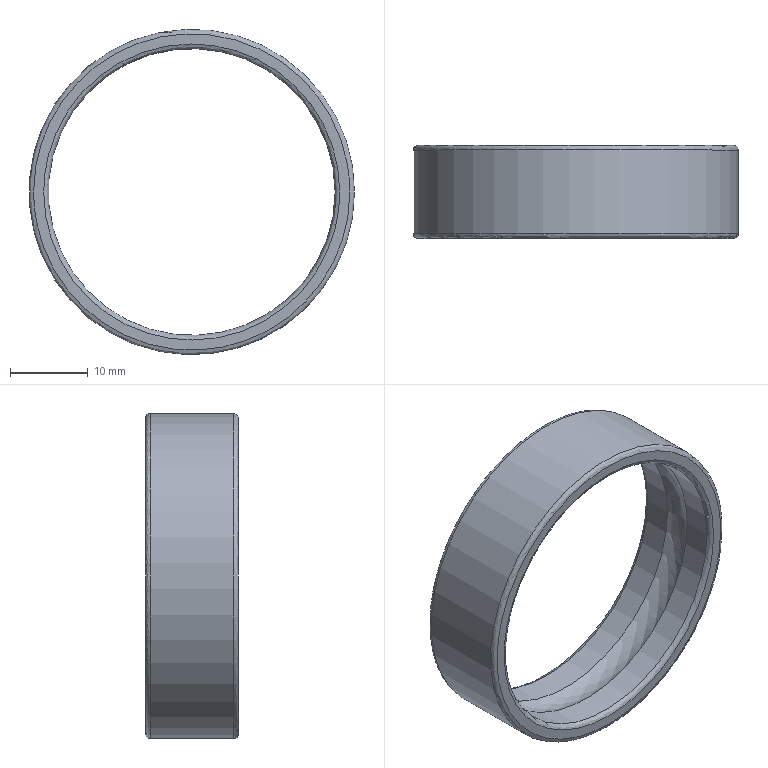Part | STEP file | BF-20_id1382_x_t | 1 solid | 10 faces | box 42 x 12 x 42 mm | volume 3541 mm3 | other 5 | cylinder 3 | plane 2 | commonest cylinder face diameters 37 x2 42 x1
STEP:
#1=CARTESIAN_POINT('',(0.,0.,0.));
#2=DIRECTION('',(0.,0.,1.));
#3=DIRECTION('',(1.,0.,0.));
#4=AXIS2_PLACEMENT_3D('',#1,#2,#3);
#5=CARTESIAN_POINT('',(-250.,-70.262,-165.5));
#6=VERTEX_POINT('',#5);
#7=CARTESIAN_POINT('',(-268.5,-70.262,-165.5));
#8=DIRECTION('',(0.,1.,0.));
#9=DIRECTION('',(1.,0.,0.));
#10=AXIS2_PLACEMENT_3D('',#7,#8,#9);
#11=CIRCLE('',#10,18.5);
#12=CARTESIAN_POINT('',(-253.,-72.064,-165.5));
#13=DIRECTION('',(0.,0.,1.));
#14=DIRECTION('',(1.,0.,0.));
#15=AXIS2_PLACEMENT_3D('',#12,#13,#14);
#16=CIRCLE('',#15,3.5);
#17=CARTESIAN_POINT('',(-268.5,-72.064,-165.5));
#18=DIRECTION('',(0.,-1.,0.));
#19=AXIS1_PLACEMENT('',#17,#18);
#20=SURFACE_OF_REVOLUTION('',#16,#19);
#21=CARTESIAN_POINT('',(6.283,6.824));
#22=DIRECTION('',(-1.,0.));
#23=VECTOR('',#22,1.);
#24=LINE('',#21,#23);
#25=(GEOMETRIC_REPRESENTATION_CONTEXT(2)PARAMETRIC_REPRESENTATION_CONTEXT()REPRESENTATION_CONTEXT('',''));
#26=DEFINITIONAL_REPRESENTATION('',(#24),#25);
#27=PCURVE('',#20,#26);
#28=CARTESIAN_POINT('',(-268.5,-80.904,-165.5));
#29=DIRECTION('',(0.,-1.,0.));
#30=DIRECTION('',(1.,0.,0.));
#31=AXIS2_PLACEMENT_3D('',#28,#29,#30);
#32=CYLINDRICAL_SURFACE('',#31,18.5);
#33=CARTESIAN_POINT('',(6.283,-10.642));
#34=DIRECTION('',(-1.,0.));
#35=VECTOR('',#34,1.);
#36=LINE('',#33,#35);
#37=(GEOMETRIC_REPRESENTATION_CONTEXT(2)PARAMETRIC_REPRESENTATION_CONTEXT()REPRESENTATION_CONTEXT('',''));
#38=DEFINITIONAL_REPRESENTATION('',(#36),#37);
#39=PCURVE('',#32,#38);
#40=SURFACE_CURVE('',#11,(#27,#39),.PCURVE_S1.);
#41=EDGE_CURVE('',#6,#6,#40,.T.);
#42=ORIENTED_EDGE('',*,*,#41,.T.);
#43=CARTESIAN_POINT('',(-250.,-73.867,-165.5));
#44=VERTEX_POINT('',#43);
#45=CARTESIAN_POINT('',(-250.,-73.867,-165.5));
#46=CARTESIAN_POINT('',(-249.675,-73.326,-165.5));
#47=CARTESIAN_POINT('',(-249.467,-72.715,-165.5));
#48=CARTESIAN_POINT('',(-249.395,-72.064,-165.5));
#49=CARTESIAN_POINT('',(-249.467,-71.414,-165.5));
#50=CARTESIAN_POINT('',(-249.675,-70.803,-165.5));
#51=CARTESIAN_POINT('',(-250.,-70.262,-165.5));
#52=B_SPLINE_CURVE_WITH_KNOTS('',6,(#45,#46,#47,#48,#49,#50,#51),.UNSPECIFIED.,.F.,.F.,(7,7),(-0.5411,0.5411),.PIECEWISE_BEZIER_KNOTS.);
#53=CARTESIAN_POINT('',(0.,6.283));
#54=DIRECTION('',(0.,1.));
#55=VECTOR('',#54,1.);
#56=LINE('',#53,#55);
#57=(GEOMETRIC_REPRESENTATION_CONTEXT(2)PARAMETRIC_REPRESENTATION_CONTEXT()REPRESENTATION_CONTEXT('',''));
#58=DEFINITIONAL_REPRESENTATION('',(#56),#57);
#59=PCURVE('',#20,#58);
#60=CARTESIAN_POINT('',(6.283,6.283));
#61=DIRECTION('',(0.,1.));
#62=VECTOR('',#61,1.);
#63=LINE('',#60,#62);
#64=(GEOMETRIC_REPRESENTATION_CONTEXT(2)PARAMETRIC_REPRESENTATION_CONTEXT()REPRESENTATION_CONTEXT('',''));
#65=DEFINITIONAL_REPRESENTATION('',(#63),#64);
#66=PCURVE('',#20,#65);
#67=SEAM_CURVE('',#52,(#59,#66),.PCURVE_S1.);
#68=EDGE_CURVE('',#44,#6,#67,.T.);
#69=ORIENTED_EDGE('',*,*,#68,.F.);
#70=CARTESIAN_POINT('',(-268.5,-73.867,-165.5));
#71=DIRECTION('',(0.,-1.,0.));
#72=DIRECTION('',(1.,0.,0.));
#73=AXIS2_PLACEMENT_3D('',#70,#71,#72);
#74=CIRCLE('',#73,18.5);
#75=CARTESIAN_POINT('',(0.,5.742));
#76=DIRECTION('',(1.,0.));
#77=VECTOR('',#76,1.);
#78=LINE('',#75,#77);
#79=(GEOMETRIC_REPRESENTATION_CONTEXT(2)PARAMETRIC_REPRESENTATION_CONTEXT()REPRESENTATION_CONTEXT('',''));
#80=DEFINITIONAL_REPRESENTATION('',(#78),#79);
#81=PCURVE('',#20,#80);
#82=CARTESIAN_POINT('',(-268.5,-80.904,-165.5));
#83=DIRECTION('',(0.,-1.,0.));
#84=DIRECTION('',(1.,0.,0.));
#85=AXIS2_PLACEMENT_3D('',#82,#83,#84);
#86=CYLINDRICAL_SURFACE('',#85,18.5);
#87=CARTESIAN_POINT('',(0.,-7.037));
#88=DIRECTION('',(1.,0.));
#89=VECTOR('',#88,1.);
#90=LINE('',#87,#89);
#91=(GEOMETRIC_REPRESENTATION_CONTEXT(2)PARAMETRIC_REPRESENTATION_CONTEXT()REPRESENTATION_CONTEXT('',''));
#92=DEFINITIONAL_REPRESENTATION('',(#90),#91);
#93=PCURVE('',#86,#92);
#94=SURFACE_CURVE('',#74,(#81,#93),.PCURVE_S1.);
#95=EDGE_CURVE('',#44,#44,#94,.T.);
#96=ORIENTED_EDGE('',*,*,#95,.T.);
#97=ORIENTED_EDGE('',*,*,#68,.T.);
#98=EDGE_LOOP('',(#42,#69,#96,#97));
#99=FACE_BOUND('',#98,.T.);
#100=ADVANCED_FACE('',(#99),#20,.T.);
#101=CARTESIAN_POINT('',(-250.,-66.664,-165.5));
#102=VERTEX_POINT('',#101);
#103=CARTESIAN_POINT('',(-268.5,-66.664,-165.5));
#104=DIRECTION('',(0.,-1.,0.));
#105=DIRECTION('',(1.,0.,0.));
#106=AXIS2_PLACEMENT_3D('',#103,#104,#105);
#107=CIRCLE('',#106,18.5);
#108=CARTESIAN_POINT('',(0.,-14.239));
#109=DIRECTION('',(1.,0.));
#110=VECTOR('',#109,1.);
#111=LINE('',#108,#110);
#112=(GEOMETRIC_REPRESENTATION_CONTEXT(2)PARAMETRIC_REPRESENTATION_CONTEXT()REPRESENTATION_CONTEXT('',''));
#113=DEFINITIONAL_REPRESENTATION('',(#111),#112);
#114=PCURVE('',#32,#113);
#115=CARTESIAN_POINT('',(-249.4,-66.664,-165.5));
#116=DIRECTION('',(0.,0.,1.));
#117=DIRECTION('',(1.,0.,0.));
#118=AXIS2_PLACEMENT_3D('',#115,#116,#117);
#119=CIRCLE('',#118,0.6);
#120=CARTESIAN_POINT('',(-268.5,-66.664,-165.5));
#121=DIRECTION('',(0.,-1.,0.));
#122=AXIS1_PLACEMENT('',#120,#121);
#123=SURFACE_OF_REVOLUTION('',#119,#122);
#124=CARTESIAN_POINT('',(0.,9.425));
#125=DIRECTION('',(1.,0.));
#126=VECTOR('',#125,1.);
#127=LINE('',#124,#126);
#128=(GEOMETRIC_REPRESENTATION_CONTEXT(2)PARAMETRIC_REPRESENTATION_CONTEXT()REPRESENTATION_CONTEXT('',''));
#129=DEFINITIONAL_REPRESENTATION('',(#127),#128);
#130=PCURVE('',#123,#129);
#131=SURFACE_CURVE('',#107,(#114,#130),.PCURVE_S1.);
#132=EDGE_CURVE('',#102,#102,#131,.T.);
#133=ORIENTED_EDGE('',*,*,#132,.T.);
#134=CARTESIAN_POINT('',(-250.,-66.664,-165.5));
#135=CARTESIAN_POINT('',(-250.,-70.262,-165.5));
#136=B_SPLINE_CURVE_WITH_KNOTS('',1,(#134,#135),.UNSPECIFIED.,.F.,.F.,(2,2),(-14.239,-10.642),.PIECEWISE_BEZIER_KNOTS.);
#137=CARTESIAN_POINT('',(6.283,0.));
#138=DIRECTION('',(0.,1.));
#139=VECTOR('',#138,1.);
#140=LINE('',#137,#139);
#141=(GEOMETRIC_REPRESENTATION_CONTEXT(2)PARAMETRIC_REPRESENTATION_CONTEXT()REPRESENTATION_CONTEXT('',''));
#142=DEFINITIONAL_REPRESENTATION('',(#140),#141);
#143=PCURVE('',#32,#142);
#144=CARTESIAN_POINT('',(0.,0.));
#145=DIRECTION('',(0.,1.));
#146=VECTOR('',#145,1.);
#147=LINE('',#144,#146);
#148=(GEOMETRIC_REPRESENTATION_CONTEXT(2)PARAMETRIC_REPRESENTATION_CONTEXT()REPRESENTATION_CONTEXT('',''));
#149=DEFINITIONAL_REPRESENTATION('',(#147),#148);
#150=PCURVE('',#32,#149);
#151=SEAM_CURVE('',#136,(#143,#150),.PCURVE_S1.);
#152=EDGE_CURVE('',#102,#6,#151,.T.);
#153=ORIENTED_EDGE('',*,*,#152,.T.);
#154=ORIENTED_EDGE('',*,*,#41,.T.);
#155=ORIENTED_EDGE('',*,*,#152,.F.);
#156=EDGE_LOOP('',(#133,#153,#154,#155));
#157=FACE_BOUND('',#156,.F.);
#158=ADVANCED_FACE('',(#157),#32,.F.);
#159=ORIENTED_EDGE('',*,*,#95,.T.);
#160=CARTESIAN_POINT('',(-250.,-77.464,-165.5));
#161=VERTEX_POINT('',#160);
#162=CARTESIAN_POINT('',(-250.,-73.867,-165.5));
#163=CARTESIAN_POINT('',(-250.,-77.464,-165.5));
#164=B_SPLINE_CURVE_WITH_KNOTS('',1,(#162,#163),.UNSPECIFIED.,.F.,.F.,(2,2),(-7.037,-3.439),.PIECEWISE_BEZIER_KNOTS.);
#165=CARTESIAN_POINT('',(6.283,0.));
#166=DIRECTION('',(0.,1.));
#167=VECTOR('',#166,1.);
#168=LINE('',#165,#167);
#169=(GEOMETRIC_REPRESENTATION_CONTEXT(2)PARAMETRIC_REPRESENTATION_CONTEXT()REPRESENTATION_CONTEXT('',''));
#170=DEFINITIONAL_REPRESENTATION('',(#168),#169);
#171=PCURVE('',#86,#170);
#172=CARTESIAN_POINT('',(0.,0.));
#173=DIRECTION('',(0.,1.));
#174=VECTOR('',#173,1.);
#175=LINE('',#172,#174);
#176=(GEOMETRIC_REPRESENTATION_CONTEXT(2)PARAMETRIC_REPRESENTATION_CONTEXT()REPRESENTATION_CONTEXT('',''));
#177=DEFINITIONAL_REPRESENTATION('',(#175),#176);
#178=PCURVE('',#86,#177);
#179=SEAM_CURVE('',#164,(#171,#178),.PCURVE_S1.);
#180=EDGE_CURVE('',#44,#161,#179,.T.);
#181=ORIENTED_EDGE('',*,*,#180,.T.);
#182=CARTESIAN_POINT('',(-268.5,-77.464,-165.5));
#183=DIRECTION('',(0.,1.,0.));
#184=DIRECTION('',(1.,0.,0.));
#185=AXIS2_PLACEMENT_3D('',#182,#183,#184);
#186=CIRCLE('',#185,18.5);
#187=CARTESIAN_POINT('',(6.283,-3.439));
#188=DIRECTION('',(-1.,0.));
#189=VECTOR('',#188,1.);
#190=LINE('',#187,#189);
#191=(GEOMETRIC_REPRESENTATION_CONTEXT(2)PARAMETRIC_REPRESENTATION_CONTEXT()REPRESENTATION_CONTEXT('',''));
#192=DEFINITIONAL_REPRESENTATION('',(#190),#191);
#193=PCURVE('',#86,#192);
#194=CARTESIAN_POINT('',(-249.4,-77.464,-165.5));
#195=DIRECTION('',(0.,0.,1.));
#196=DIRECTION('',(1.,0.,0.));
#197=AXIS2_PLACEMENT_3D('',#194,#195,#196);
#198=CIRCLE('',#197,0.6);
#199=CARTESIAN_POINT('',(-268.5,-77.464,-165.5));
#200=DIRECTION('',(0.,-1.,0.));
#201=AXIS1_PLACEMENT('',#199,#200);
#202=SURFACE_OF_REVOLUTION('',#198,#201);
#203=CARTESIAN_POINT('',(6.283,3.142));
#204=DIRECTION('',(-1.,0.));
#205=VECTOR('',#204,1.);
#206=LINE('',#203,#205);
#207=(GEOMETRIC_REPRESENTATION_CONTEXT(2)PARAMETRIC_REPRESENTATION_CONTEXT()REPRESENTATION_CONTEXT('',''));
#208=DEFINITIONAL_REPRESENTATION('',(#206),#207);
#209=PCURVE('',#202,#208);
#210=SURFACE_CURVE('',#186,(#193,#209),.PCURVE_S1.);
#211=EDGE_CURVE('',#161,#161,#210,.T.);
#212=ORIENTED_EDGE('',*,*,#211,.T.);
#213=ORIENTED_EDGE('',*,*,#180,.F.);
#214=EDGE_LOOP('',(#159,#181,#212,#213));
#215=FACE_BOUND('',#214,.F.);
#216=ADVANCED_FACE('',(#215),#86,.F.);
#217=CARTESIAN_POINT('',(-287.6,-66.064,-165.5));
#218=VERTEX_POINT('',#217);
#219=CARTESIAN_POINT('',(-249.4,-66.064,-165.5));
#220=VERTEX_POINT('',#219);
#221=CARTESIAN_POINT('',(-287.6,-66.064,-165.5));
#222=CARTESIAN_POINT('',(-287.6,-66.064,-127.3));
#223=CARTESIAN_POINT('',(-249.4,-66.064,-127.3));
#224=CARTESIAN_POINT('',(-249.4,-66.064,-165.5));
#225=(BOUNDED_CURVE()B_SPLINE_CURVE(3,(#221,#222,#223,#224),.UNSPECIFIED.,.F.,.F.)B_SPLINE_CURVE_WITH_KNOTS((4,4),(0.,1.),.PIECEWISE_BEZIER_KNOTS.)CURVE()GEOMETRIC_REPRESENTATION_ITEM()RATIONAL_B_SPLINE_CURVE((1.,0.3333,0.3333,1.))REPRESENTATION_ITEM(''));
#226=CARTESIAN_POINT('',(3.142,7.854));
#227=CARTESIAN_POINT('',(3.111,7.854));
#228=CARTESIAN_POINT('',(3.048,7.854));
#229=CARTESIAN_POINT('',(2.944,7.854));
#230=CARTESIAN_POINT('',(2.83,7.854));
#231=CARTESIAN_POINT('',(2.706,7.854));
#232=CARTESIAN_POINT('',(2.571,7.854));
#233=CARTESIAN_POINT('',(2.426,7.854));
#234=CARTESIAN_POINT('',(2.27,7.854));
#235=CARTESIAN_POINT('',(2.105,7.854));
#236=CARTESIAN_POINT('',(1.931,7.854));
#237=CARTESIAN_POINT('',(1.753,7.854));
#238=CARTESIAN_POINT('',(1.571,7.854));
#239=CARTESIAN_POINT('',(1.389,7.854));
#240=CARTESIAN_POINT('',(1.21,7.854));
#241=CARTESIAN_POINT('',(1.037,7.854));
#242=CARTESIAN_POINT('',(0.8717,7.854));
#243=CARTESIAN_POINT('',(0.7158,7.854));
#244=CARTESIAN_POINT('',(0.5703,7.854));
#245=CARTESIAN_POINT('',(0.4356,7.854));
#246=CARTESIAN_POINT('',(0.3115,7.854));
#247=CARTESIAN_POINT('',(0.1977,7.854));
#248=CARTESIAN_POINT('',(0.09367,7.854));
#249=CARTESIAN_POINT('',(0.0303,7.854));
#250=CARTESIAN_POINT('',(0.,7.854));
#251=B_SPLINE_CURVE_WITH_KNOTS('',3,(#226,#227,#228,#229,#230,#231,#232,#233,#234,#235,#236,#237,#238,#239,#240,#241,#242,#243,#244,#245,#246,#247,#248,#249,#250),.UNSPECIFIED.,.F.,.F.,(4,1,1,1,1,1,1,1,1,1,1,1,1,1,1,1,1,1,1,1,1,1,4),(0.,0.04545,0.09091,0.1364,0.1818,0.2273,0.2727,0.3182,0.3636,0.4091,0.4545,0.5,0.5455,0.5909,0.6364,0.6818,0.7273,0.7727,0.8182,0.8636,0.9091,0.9545,1.),.QUASI_UNIFORM_KNOTS.);
#252=(GEOMETRIC_REPRESENTATION_CONTEXT(2)PARAMETRIC_REPRESENTATION_CONTEXT()REPRESENTATION_CONTEXT('',''));
#253=DEFINITIONAL_REPRESENTATION('',(#251),#252);
#254=PCURVE('',#123,#253);
#255=CARTESIAN_POINT('',(-268.5,-66.064,-145.1));
#256=DIRECTION('',(0.,-1.,0.));
#257=DIRECTION('',(1.,0.,0.));
#258=AXIS2_PLACEMENT_3D('',#255,#256,#257);
#259=PLANE('',#258);
#260=CARTESIAN_POINT('',(-19.1,-20.4));
#261=CARTESIAN_POINT('',(-19.1,17.8));
#262=CARTESIAN_POINT('',(19.1,17.8));
#263=CARTESIAN_POINT('',(19.1,-20.4));
#264=(BOUNDED_CURVE()B_SPLINE_CURVE(3,(#260,#261,#262,#263),.UNSPECIFIED.,.F.,.F.)B_SPLINE_CURVE_WITH_KNOTS((4,4),(0.,1.),.PIECEWISE_BEZIER_KNOTS.)CURVE()GEOMETRIC_REPRESENTATION_ITEM()RATIONAL_B_SPLINE_CURVE((1.,0.3333,0.3333,1.))REPRESENTATION_ITEM(''));
#265=(GEOMETRIC_REPRESENTATION_CONTEXT(2)PARAMETRIC_REPRESENTATION_CONTEXT()REPRESENTATION_CONTEXT('',''));
#266=DEFINITIONAL_REPRESENTATION('',(#264),#265);
#267=PCURVE('',#259,#266);
#268=SURFACE_CURVE('',#225,(#254,#267),.PCURVE_S1.);
#269=EDGE_CURVE('',#218,#220,#268,.T.);
#270=ORIENTED_EDGE('',*,*,#269,.F.);
#271=CARTESIAN_POINT('',(-249.4,-66.064,-165.5));
#272=CARTESIAN_POINT('',(-249.4,-66.064,-203.7));
#273=CARTESIAN_POINT('',(-287.6,-66.064,-203.7));
#274=CARTESIAN_POINT('',(-287.6,-66.064,-165.5));
#275=(BOUNDED_CURVE()B_SPLINE_CURVE(3,(#271,#272,#273,#274),.UNSPECIFIED.,.F.,.F.)B_SPLINE_CURVE_WITH_KNOTS((4,4),(0.,1.),.PIECEWISE_BEZIER_KNOTS.)CURVE()GEOMETRIC_REPRESENTATION_ITEM()RATIONAL_B_SPLINE_CURVE((1.,0.3333,0.3333,1.))REPRESENTATION_ITEM(''));
#276=CARTESIAN_POINT('',(6.283,7.854));
#277=CARTESIAN_POINT('',(6.253,7.854));
#278=CARTESIAN_POINT('',(6.19,7.854));
#279=CARTESIAN_POINT('',(6.085,7.854));
#280=CARTESIAN_POINT('',(5.972,7.854));
#281=CARTESIAN_POINT('',(5.848,7.854));
#282=CARTESIAN_POINT('',(5.713,7.854));
#283=CARTESIAN_POINT('',(5.567,7.854));
#284=CARTESIAN_POINT('',(5.412,7.854));
#285=CARTESIAN_POINT('',(5.246,7.854));
#286=CARTESIAN_POINT('',(5.073,7.854));
#287=CARTESIAN_POINT('',(4.894,7.854));
#288=CARTESIAN_POINT('',(4.712,7.854));
#289=CARTESIAN_POINT('',(4.531,7.854));
#290=CARTESIAN_POINT('',(4.352,7.854));
#291=CARTESIAN_POINT('',(4.179,7.854));
#292=CARTESIAN_POINT('',(4.013,7.854));
#293=CARTESIAN_POINT('',(3.857,7.854));
#294=CARTESIAN_POINT('',(3.712,7.854));
#295=CARTESIAN_POINT('',(3.577,7.854));
#296=CARTESIAN_POINT('',(3.453,7.854));
#297=CARTESIAN_POINT('',(3.339,7.854));
#298=CARTESIAN_POINT('',(3.235,7.854));
#299=CARTESIAN_POINT('',(3.172,7.854));
#300=CARTESIAN_POINT('',(3.142,7.854));
#301=B_SPLINE_CURVE_WITH_KNOTS('',3,(#276,#277,#278,#279,#280,#281,#282,#283,#284,#285,#286,#287,#288,#289,#290,#291,#292,#293,#294,#295,#296,#297,#298,#299,#300),.UNSPECIFIED.,.F.,.F.,(4,1,1,1,1,1,1,1,1,1,1,1,1,1,1,1,1,1,1,1,1,1,4),(0.,0.04545,0.09091,0.1364,0.1818,0.2273,0.2727,0.3182,0.3636,0.4091,0.4545,0.5,0.5455,0.5909,0.6364,0.6818,0.7273,0.7727,0.8182,0.8636,0.9091,0.9545,1.),.QUASI_UNIFORM_KNOTS.);
#302=(GEOMETRIC_REPRESENTATION_CONTEXT(2)PARAMETRIC_REPRESENTATION_CONTEXT()REPRESENTATION_CONTEXT('',''));
#303=DEFINITIONAL_REPRESENTATION('',(#301),#302);
#304=PCURVE('',#123,#303);
#305=CARTESIAN_POINT('',(19.1,-20.4));
#306=CARTESIAN_POINT('',(19.1,-58.6));
#307=CARTESIAN_POINT('',(-19.1,-58.6));
#308=CARTESIAN_POINT('',(-19.1,-20.4));
#309=(BOUNDED_CURVE()B_SPLINE_CURVE(3,(#305,#306,#307,#308),.UNSPECIFIED.,.F.,.F.)B_SPLINE_CURVE_WITH_KNOTS((4,4),(0.,1.),.PIECEWISE_BEZIER_KNOTS.)CURVE()GEOMETRIC_REPRESENTATION_ITEM()RATIONAL_B_SPLINE_CURVE((1.,0.3333,0.3333,1.))REPRESENTATION_ITEM(''));
#310=(GEOMETRIC_REPRESENTATION_CONTEXT(2)PARAMETRIC_REPRESENTATION_CONTEXT()REPRESENTATION_CONTEXT('',''));
#311=DEFINITIONAL_REPRESENTATION('',(#309),#310);
#312=PCURVE('',#259,#311);
#313=SURFACE_CURVE('',#275,(#304,#312),.PCURVE_S1.);
#314=EDGE_CURVE('',#220,#218,#313,.T.);
#315=ORIENTED_EDGE('',*,*,#314,.F.);
#316=CARTESIAN_POINT('',(-249.4,-66.064,-165.5));
#317=CARTESIAN_POINT('',(-249.56,-66.064,-165.5));
#318=CARTESIAN_POINT('',(-249.717,-66.115,-165.5));
#319=CARTESIAN_POINT('',(-249.851,-66.213,-165.5));
#320=CARTESIAN_POINT('',(-249.949,-66.348,-165.5));
#321=CARTESIAN_POINT('',(-250.,-66.504,-165.5));
#322=CARTESIAN_POINT('',(-250.,-66.664,-165.5));
#323=(BOUNDED_CURVE()B_SPLINE_CURVE(6,(#316,#317,#318,#319,#320,#321,#322),.UNSPECIFIED.,.F.,.F.)B_SPLINE_CURVE_WITH_KNOTS((7,7),(1.571,3.142),.PIECEWISE_BEZIER_KNOTS.)CURVE()GEOMETRIC_REPRESENTATION_ITEM()RATIONAL_B_SPLINE_CURVE((1.031,1.01,0.9979,0.994,0.9979,1.01,1.031))REPRESENTATION_ITEM(''));
#324=CARTESIAN_POINT('',(6.283,6.283));
#325=DIRECTION('',(0.,1.));
#326=VECTOR('',#325,1.);
#327=LINE('',#324,#326);
#328=(GEOMETRIC_REPRESENTATION_CONTEXT(2)PARAMETRIC_REPRESENTATION_CONTEXT()REPRESENTATION_CONTEXT('',''));
#329=DEFINITIONAL_REPRESENTATION('',(#327),#328);
#330=PCURVE('',#123,#329);
#331=CARTESIAN_POINT('',(0.,6.283));
#332=DIRECTION('',(0.,1.));
#333=VECTOR('',#332,1.);
#334=LINE('',#331,#333);
#335=(GEOMETRIC_REPRESENTATION_CONTEXT(2)PARAMETRIC_REPRESENTATION_CONTEXT()REPRESENTATION_CONTEXT('',''));
#336=DEFINITIONAL_REPRESENTATION('',(#334),#335);
#337=PCURVE('',#123,#336);
#338=SEAM_CURVE('',#323,(#330,#337),.PCURVE_S1.);
#339=EDGE_CURVE('',#220,#102,#338,.T.);
#340=ORIENTED_EDGE('',*,*,#339,.T.);
#341=ORIENTED_EDGE('',*,*,#132,.F.);
#342=ORIENTED_EDGE('',*,*,#339,.F.);
#343=EDGE_LOOP('',(#270,#315,#340,#341,#342));
#344=FACE_BOUND('',#343,.F.);
#345=ADVANCED_FACE('',(#344),#123,.F.);
#346=ORIENTED_EDGE('',*,*,#211,.F.);
#347=CARTESIAN_POINT('',(-249.4,-78.064,-165.5));
#348=VERTEX_POINT('',#347);
#349=CARTESIAN_POINT('',(-250.,-77.464,-165.5));
#350=CARTESIAN_POINT('',(-250.,-77.625,-165.5));
#351=CARTESIAN_POINT('',(-249.949,-77.781,-165.5));
#352=CARTESIAN_POINT('',(-249.851,-77.916,-165.5));
#353=CARTESIAN_POINT('',(-249.717,-78.013,-165.5));
#354=CARTESIAN_POINT('',(-249.56,-78.064,-165.5));
#355=CARTESIAN_POINT('',(-249.4,-78.064,-165.5));
#356=(BOUNDED_CURVE()B_SPLINE_CURVE(6,(#349,#350,#351,#352,#353,#354,#355),.UNSPECIFIED.,.F.,.F.)B_SPLINE_CURVE_WITH_KNOTS((7,7),(3.142,4.712),.PIECEWISE_BEZIER_KNOTS.)CURVE()GEOMETRIC_REPRESENTATION_ITEM()RATIONAL_B_SPLINE_CURVE((1.031,1.01,0.9979,0.994,0.9979,1.01,1.031))REPRESENTATION_ITEM(''));
#357=CARTESIAN_POINT('',(6.283,0.));
#358=DIRECTION('',(0.,1.));
#359=VECTOR('',#358,1.);
#360=LINE('',#357,#359);
#361=(GEOMETRIC_REPRESENTATION_CONTEXT(2)PARAMETRIC_REPRESENTATION_CONTEXT()REPRESENTATION_CONTEXT('',''));
#362=DEFINITIONAL_REPRESENTATION('',(#360),#361);
#363=PCURVE('',#202,#362);
#364=CARTESIAN_POINT('',(0.,0.));
#365=DIRECTION('',(0.,1.));
#366=VECTOR('',#365,1.);
#367=LINE('',#364,#366);
#368=(GEOMETRIC_REPRESENTATION_CONTEXT(2)PARAMETRIC_REPRESENTATION_CONTEXT()REPRESENTATION_CONTEXT('',''));
#369=DEFINITIONAL_REPRESENTATION('',(#367),#368);
#370=PCURVE('',#202,#369);
#371=SEAM_CURVE('',#356,(#363,#370),.PCURVE_S1.);
#372=EDGE_CURVE('',#161,#348,#371,.T.);
#373=ORIENTED_EDGE('',*,*,#372,.T.);
#374=CARTESIAN_POINT('',(-287.6,-78.064,-165.5));
#375=VERTEX_POINT('',#374);
#376=CARTESIAN_POINT('',(-287.6,-78.064,-165.5));
#377=CARTESIAN_POINT('',(-287.6,-78.064,-203.7));
#378=CARTESIAN_POINT('',(-249.4,-78.064,-203.7));
#379=CARTESIAN_POINT('',(-249.4,-78.064,-165.5));
#380=(BOUNDED_CURVE()B_SPLINE_CURVE(3,(#376,#377,#378,#379),.UNSPECIFIED.,.F.,.F.)B_SPLINE_CURVE_WITH_KNOTS((4,4),(0.,1.),.PIECEWISE_BEZIER_KNOTS.)CURVE()GEOMETRIC_REPRESENTATION_ITEM()RATIONAL_B_SPLINE_CURVE((1.,0.3333,0.3333,1.))REPRESENTATION_ITEM(''));
#381=CARTESIAN_POINT('',(3.142,4.712));
#382=CARTESIAN_POINT('',(3.172,4.712));
#383=CARTESIAN_POINT('',(3.235,4.712));
#384=CARTESIAN_POINT('',(3.339,4.712));
#385=CARTESIAN_POINT('',(3.453,4.712));
#386=CARTESIAN_POINT('',(3.577,4.712));
#387=CARTESIAN_POINT('',(3.712,4.712));
#388=CARTESIAN_POINT('',(3.857,4.712));
#389=CARTESIAN_POINT('',(4.013,4.712));
#390=CARTESIAN_POINT('',(4.179,4.712));
#391=CARTESIAN_POINT('',(4.352,4.712));
#392=CARTESIAN_POINT('',(4.531,4.712));
#393=CARTESIAN_POINT('',(4.712,4.712));
#394=CARTESIAN_POINT('',(4.894,4.712));
#395=CARTESIAN_POINT('',(5.073,4.712));
#396=CARTESIAN_POINT('',(5.246,4.712));
#397=CARTESIAN_POINT('',(5.412,4.712));
#398=CARTESIAN_POINT('',(5.567,4.712));
#399=CARTESIAN_POINT('',(5.713,4.712));
#400=CARTESIAN_POINT('',(5.848,4.712));
#401=CARTESIAN_POINT('',(5.972,4.712));
#402=CARTESIAN_POINT('',(6.085,4.712));
#403=CARTESIAN_POINT('',(6.19,4.712));
#404=CARTESIAN_POINT('',(6.253,4.712));
#405=CARTESIAN_POINT('',(6.283,4.712));
#406=B_SPLINE_CURVE_WITH_KNOTS('',3,(#381,#382,#383,#384,#385,#386,#387,#388,#389,#390,#391,#392,#393,#394,#395,#396,#397,#398,#399,#400,#401,#402,#403,#404,#405),.UNSPECIFIED.,.F.,.F.,(4,1,1,1,1,1,1,1,1,1,1,1,1,1,1,1,1,1,1,1,1,1,4),(0.,0.04545,0.09091,0.1364,0.1818,0.2273,0.2727,0.3182,0.3636,0.4091,0.4545,0.5,0.5455,0.5909,0.6364,0.6818,0.7273,0.7727,0.8182,0.8636,0.9091,0.9545,1.),.QUASI_UNIFORM_KNOTS.);
#407=(GEOMETRIC_REPRESENTATION_CONTEXT(2)PARAMETRIC_REPRESENTATION_CONTEXT()REPRESENTATION_CONTEXT('',''));
#408=DEFINITIONAL_REPRESENTATION('',(#406),#407);
#409=PCURVE('',#202,#408);
#410=CARTESIAN_POINT('',(-268.5,-78.064,-145.1));
#411=DIRECTION('',(0.,1.,0.));
#412=DIRECTION('',(-1.,0.,0.));
#413=AXIS2_PLACEMENT_3D('',#410,#411,#412);
#414=PLANE('',#413);
#415=CARTESIAN_POINT('',(19.1,-20.4));
#416=CARTESIAN_POINT('',(19.1,-58.6));
#417=CARTESIAN_POINT('',(-19.1,-58.6));
#418=CARTESIAN_POINT('',(-19.1,-20.4));
#419=(BOUNDED_CURVE()B_SPLINE_CURVE(3,(#415,#416,#417,#418),.UNSPECIFIED.,.F.,.F.)B_SPLINE_CURVE_WITH_KNOTS((4,4),(0.,1.),.PIECEWISE_BEZIER_KNOTS.)CURVE()GEOMETRIC_REPRESENTATION_ITEM()RATIONAL_B_SPLINE_CURVE((1.,0.3333,0.3333,1.))REPRESENTATION_ITEM(''));
#420=(GEOMETRIC_REPRESENTATION_CONTEXT(2)PARAMETRIC_REPRESENTATION_CONTEXT()REPRESENTATION_CONTEXT('',''));
#421=DEFINITIONAL_REPRESENTATION('',(#419),#420);
#422=PCURVE('',#414,#421);
#423=SURFACE_CURVE('',#380,(#409,#422),.PCURVE_S1.);
#424=EDGE_CURVE('',#375,#348,#423,.T.);
#425=ORIENTED_EDGE('',*,*,#424,.F.);
#426=CARTESIAN_POINT('',(-249.4,-78.064,-165.5));
#427=CARTESIAN_POINT('',(-249.4,-78.064,-127.3));
#428=CARTESIAN_POINT('',(-287.6,-78.064,-127.3));
#429=CARTESIAN_POINT('',(-287.6,-78.064,-165.5));
#430=(BOUNDED_CURVE()B_SPLINE_CURVE(3,(#426,#427,#428,#429),.UNSPECIFIED.,.F.,.F.)B_SPLINE_CURVE_WITH_KNOTS((4,4),(0.,1.),.PIECEWISE_BEZIER_KNOTS.)CURVE()GEOMETRIC_REPRESENTATION_ITEM()RATIONAL_B_SPLINE_CURVE((1.,0.3333,0.3333,1.))REPRESENTATION_ITEM(''));
#431=CARTESIAN_POINT('',(0.,4.712));
#432=CARTESIAN_POINT('',(0.0303,4.712));
#433=CARTESIAN_POINT('',(0.09367,4.712));
#434=CARTESIAN_POINT('',(0.1977,4.712));
#435=CARTESIAN_POINT('',(0.3115,4.712));
#436=CARTESIAN_POINT('',(0.4356,4.712));
#437=CARTESIAN_POINT('',(0.5703,4.712));
#438=CARTESIAN_POINT('',(0.7158,4.712));
#439=CARTESIAN_POINT('',(0.8717,4.712));
#440=CARTESIAN_POINT('',(1.037,4.712));
#441=CARTESIAN_POINT('',(1.21,4.712));
#442=CARTESIAN_POINT('',(1.389,4.712));
#443=CARTESIAN_POINT('',(1.571,4.712));
#444=CARTESIAN_POINT('',(1.753,4.712));
#445=CARTESIAN_POINT('',(1.931,4.712));
#446=CARTESIAN_POINT('',(2.105,4.712));
#447=CARTESIAN_POINT('',(2.27,4.712));
#448=CARTESIAN_POINT('',(2.426,4.712));
#449=CARTESIAN_POINT('',(2.571,4.712));
#450=CARTESIAN_POINT('',(2.706,4.712));
#451=CARTESIAN_POINT('',(2.83,4.712));
#452=CARTESIAN_POINT('',(2.944,4.712));
#453=CARTESIAN_POINT('',(3.048,4.712));
#454=CARTESIAN_POINT('',(3.111,4.712));
#455=CARTESIAN_POINT('',(3.142,4.712));
#456=B_SPLINE_CURVE_WITH_KNOTS('',3,(#431,#432,#433,#434,#435,#436,#437,#438,#439,#440,#441,#442,#443,#444,#445,#446,#447,#448,#449,#450,#451,#452,#453,#454,#455),.UNSPECIFIED.,.F.,.F.,(4,1,1,1,1,1,1,1,1,1,1,1,1,1,1,1,1,1,1,1,1,1,4),(0.,0.04545,0.09091,0.1364,0.1818,0.2273,0.2727,0.3182,0.3636,0.4091,0.4545,0.5,0.5455,0.5909,0.6364,0.6818,0.7273,0.7727,0.8182,0.8636,0.9091,0.9545,1.),.QUASI_UNIFORM_KNOTS.);
#457=(GEOMETRIC_REPRESENTATION_CONTEXT(2)PARAMETRIC_REPRESENTATION_CONTEXT()REPRESENTATION_CONTEXT('',''));
#458=DEFINITIONAL_REPRESENTATION('',(#456),#457);
#459=PCURVE('',#202,#458);
#460=CARTESIAN_POINT('',(-19.1,-20.4));
#461=CARTESIAN_POINT('',(-19.1,17.8));
#462=CARTESIAN_POINT('',(19.1,17.8));
#463=CARTESIAN_POINT('',(19.1,-20.4));
#464=(BOUNDED_CURVE()B_SPLINE_CURVE(3,(#460,#461,#462,#463),.UNSPECIFIED.,.F.,.F.)B_SPLINE_CURVE_WITH_KNOTS((4,4),(0.,1.),.PIECEWISE_BEZIER_KNOTS.)CURVE()GEOMETRIC_REPRESENTATION_ITEM()RATIONAL_B_SPLINE_CURVE((1.,0.3333,0.3333,1.))REPRESENTATION_ITEM(''));
#465=(GEOMETRIC_REPRESENTATION_CONTEXT(2)PARAMETRIC_REPRESENTATION_CONTEXT()REPRESENTATION_CONTEXT('',''));
#466=DEFINITIONAL_REPRESENTATION('',(#464),#465);
#467=PCURVE('',#414,#466);
#468=SURFACE_CURVE('',#430,(#459,#467),.PCURVE_S1.);
#469=EDGE_CURVE('',#348,#375,#468,.T.);
#470=ORIENTED_EDGE('',*,*,#469,.F.);
#471=ORIENTED_EDGE('',*,*,#372,.F.);
#472=EDGE_LOOP('',(#346,#373,#425,#470,#471));
#473=FACE_BOUND('',#472,.F.);
#474=ADVANCED_FACE('',(#473),#202,.F.);
#475=ORIENTED_EDGE('',*,*,#314,.F.);
#476=ORIENTED_EDGE('',*,*,#269,.F.);
#477=EDGE_LOOP('',(#475,#476));
#478=FACE_BOUND('',#477,.T.);
#479=CARTESIAN_POINT('',(-288.9,-66.064,-165.5));
#480=VERTEX_POINT('',#479);
#481=CARTESIAN_POINT('',(-248.1,-66.064,-165.5));
#482=VERTEX_POINT('',#481);
#483=CARTESIAN_POINT('',(-288.9,-66.064,-165.5));
#484=CARTESIAN_POINT('',(-288.9,-66.064,-206.3));
#485=CARTESIAN_POINT('',(-248.1,-66.064,-206.3));
#486=CARTESIAN_POINT('',(-248.1,-66.064,-165.5));
#487=(BOUNDED_CURVE()B_SPLINE_CURVE(3,(#483,#484,#485,#486),.UNSPECIFIED.,.F.,.F.)B_SPLINE_CURVE_WITH_KNOTS((4,4),(0.,1.),.PIECEWISE_BEZIER_KNOTS.)CURVE()GEOMETRIC_REPRESENTATION_ITEM()RATIONAL_B_SPLINE_CURVE((1.,0.3333,0.3333,1.))REPRESENTATION_ITEM(''));
#488=CARTESIAN_POINT('',(-20.4,-20.4));
#489=CARTESIAN_POINT('',(-20.4,-61.2));
#490=CARTESIAN_POINT('',(20.4,-61.2));
#491=CARTESIAN_POINT('',(20.4,-20.4));
#492=(BOUNDED_CURVE()B_SPLINE_CURVE(3,(#488,#489,#490,#491),.UNSPECIFIED.,.F.,.F.)B_SPLINE_CURVE_WITH_KNOTS((4,4),(0.,1.),.PIECEWISE_BEZIER_KNOTS.)CURVE()GEOMETRIC_REPRESENTATION_ITEM()RATIONAL_B_SPLINE_CURVE((1.,0.3333,0.3333,1.))REPRESENTATION_ITEM(''));
#493=(GEOMETRIC_REPRESENTATION_CONTEXT(2)PARAMETRIC_REPRESENTATION_CONTEXT()REPRESENTATION_CONTEXT('',''));
#494=DEFINITIONAL_REPRESENTATION('',(#492),#493);
#495=PCURVE('',#259,#494);
#496=CARTESIAN_POINT('',(-248.1,-66.664,-165.5));
#497=DIRECTION('',(0.,0.,1.));
#498=DIRECTION('',(1.,0.,0.));
#499=AXIS2_PLACEMENT_3D('',#496,#497,#498);
#500=CIRCLE('',#499,0.6);
#501=CARTESIAN_POINT('',(-268.5,-66.664,-165.5));
#502=DIRECTION('',(0.,-1.,0.));
#503=AXIS1_PLACEMENT('',#501,#502);
#504=SURFACE_OF_REVOLUTION('',#500,#503);
#505=CARTESIAN_POINT('',(3.142,7.854));
#506=CARTESIAN_POINT('',(3.172,7.854));
#507=CARTESIAN_POINT('',(3.235,7.854));
#508=CARTESIAN_POINT('',(3.339,7.854));
#509=CARTESIAN_POINT('',(3.453,7.854));
#510=CARTESIAN_POINT('',(3.577,7.854));
#511=CARTESIAN_POINT('',(3.712,7.854));
#512=CARTESIAN_POINT('',(3.857,7.854));
#513=CARTESIAN_POINT('',(4.013,7.854));
#514=CARTESIAN_POINT('',(4.179,7.854));
#515=CARTESIAN_POINT('',(4.352,7.854));
#516=CARTESIAN_POINT('',(4.531,7.854));
#517=CARTESIAN_POINT('',(4.712,7.854));
#518=CARTESIAN_POINT('',(4.894,7.854));
#519=CARTESIAN_POINT('',(5.073,7.854));
#520=CARTESIAN_POINT('',(5.246,7.854));
#521=CARTESIAN_POINT('',(5.412,7.854));
#522=CARTESIAN_POINT('',(5.567,7.854));
#523=CARTESIAN_POINT('',(5.713,7.854));
#524=CARTESIAN_POINT('',(5.848,7.854));
#525=CARTESIAN_POINT('',(5.972,7.854));
#526=CARTESIAN_POINT('',(6.085,7.854));
#527=CARTESIAN_POINT('',(6.19,7.854));
#528=CARTESIAN_POINT('',(6.253,7.854));
#529=CARTESIAN_POINT('',(6.283,7.854));
#530=B_SPLINE_CURVE_WITH_KNOTS('',3,(#505,#506,#507,#508,#509,#510,#511,#512,#513,#514,#515,#516,#517,#518,#519,#520,#521,#522,#523,#524,#525,#526,#527,#528,#529),.UNSPECIFIED.,.F.,.F.,(4,1,1,1,1,1,1,1,1,1,1,1,1,1,1,1,1,1,1,1,1,1,4),(0.,0.04545,0.09091,0.1364,0.1818,0.2273,0.2727,0.3182,0.3636,0.4091,0.4545,0.5,0.5455,0.5909,0.6364,0.6818,0.7273,0.7727,0.8182,0.8636,0.9091,0.9545,1.),.QUASI_UNIFORM_KNOTS.);
#531=(GEOMETRIC_REPRESENTATION_CONTEXT(2)PARAMETRIC_REPRESENTATION_CONTEXT()REPRESENTATION_CONTEXT('',''));
#532=DEFINITIONAL_REPRESENTATION('',(#530),#531);
#533=PCURVE('',#504,#532);
#534=SURFACE_CURVE('',#487,(#495,#533),.PCURVE_S1.);
#535=EDGE_CURVE('',#480,#482,#534,.T.);
#536=ORIENTED_EDGE('',*,*,#535,.F.);
#537=CARTESIAN_POINT('',(-248.1,-66.064,-165.5));
#538=CARTESIAN_POINT('',(-248.1,-66.064,-124.7));
#539=CARTESIAN_POINT('',(-288.9,-66.064,-124.7));
#540=CARTESIAN_POINT('',(-288.9,-66.064,-165.5));
#541=(BOUNDED_CURVE()B_SPLINE_CURVE(3,(#537,#538,#539,#540),.UNSPECIFIED.,.F.,.F.)B_SPLINE_CURVE_WITH_KNOTS((4,4),(0.,1.),.PIECEWISE_BEZIER_KNOTS.)CURVE()GEOMETRIC_REPRESENTATION_ITEM()RATIONAL_B_SPLINE_CURVE((1.,0.3333,0.3333,1.))REPRESENTATION_ITEM(''));
#542=CARTESIAN_POINT('',(20.4,-20.4));
#543=CARTESIAN_POINT('',(20.4,20.4));
#544=CARTESIAN_POINT('',(-20.4,20.4));
#545=CARTESIAN_POINT('',(-20.4,-20.4));
#546=(BOUNDED_CURVE()B_SPLINE_CURVE(3,(#542,#543,#544,#545),.UNSPECIFIED.,.F.,.F.)B_SPLINE_CURVE_WITH_KNOTS((4,4),(0.,1.),.PIECEWISE_BEZIER_KNOTS.)CURVE()GEOMETRIC_REPRESENTATION_ITEM()RATIONAL_B_SPLINE_CURVE((1.,0.3333,0.3333,1.))REPRESENTATION_ITEM(''));
#547=(GEOMETRIC_REPRESENTATION_CONTEXT(2)PARAMETRIC_REPRESENTATION_CONTEXT()REPRESENTATION_CONTEXT('',''));
#548=DEFINITIONAL_REPRESENTATION('',(#546),#547);
#549=PCURVE('',#259,#548);
#550=CARTESIAN_POINT('',(0.,7.854));
#551=CARTESIAN_POINT('',(0.0303,7.854));
#552=CARTESIAN_POINT('',(0.09367,7.854));
#553=CARTESIAN_POINT('',(0.1977,7.854));
#554=CARTESIAN_POINT('',(0.3115,7.854));
#555=CARTESIAN_POINT('',(0.4356,7.854));
#556=CARTESIAN_POINT('',(0.5703,7.854));
#557=CARTESIAN_POINT('',(0.7158,7.854));
#558=CARTESIAN_POINT('',(0.8717,7.854));
#559=CARTESIAN_POINT('',(1.037,7.854));
#560=CARTESIAN_POINT('',(1.21,7.854));
#561=CARTESIAN_POINT('',(1.389,7.854));
#562=CARTESIAN_POINT('',(1.571,7.854));
#563=CARTESIAN_POINT('',(1.753,7.854));
#564=CARTESIAN_POINT('',(1.931,7.854));
#565=CARTESIAN_POINT('',(2.105,7.854));
#566=CARTESIAN_POINT('',(2.27,7.854));
#567=CARTESIAN_POINT('',(2.426,7.854));
#568=CARTESIAN_POINT('',(2.571,7.854));
#569=CARTESIAN_POINT('',(2.706,7.854));
#570=CARTESIAN_POINT('',(2.83,7.854));
#571=CARTESIAN_POINT('',(2.944,7.854));
#572=CARTESIAN_POINT('',(3.048,7.854));
#573=CARTESIAN_POINT('',(3.111,7.854));
#574=CARTESIAN_POINT('',(3.142,7.854));
#575=B_SPLINE_CURVE_WITH_KNOTS('',3,(#550,#551,#552,#553,#554,#555,#556,#557,#558,#559,#560,#561,#562,#563,#564,#565,#566,#567,#568,#569,#570,#571,#572,#573,#574),.UNSPECIFIED.,.F.,.F.,(4,1,1,1,1,1,1,1,1,1,1,1,1,1,1,1,1,1,1,1,1,1,4),(0.,0.04545,0.09091,0.1364,0.1818,0.2273,0.2727,0.3182,0.3636,0.4091,0.4545,0.5,0.5455,0.5909,0.6364,0.6818,0.7273,0.7727,0.8182,0.8636,0.9091,0.9545,1.),.QUASI_UNIFORM_KNOTS.);
#576=(GEOMETRIC_REPRESENTATION_CONTEXT(2)PARAMETRIC_REPRESENTATION_CONTEXT()REPRESENTATION_CONTEXT('',''));
#577=DEFINITIONAL_REPRESENTATION('',(#575),#576);
#578=PCURVE('',#504,#577);
#579=SURFACE_CURVE('',#541,(#549,#578),.PCURVE_S1.);
#580=EDGE_CURVE('',#482,#480,#579,.T.);
#581=ORIENTED_EDGE('',*,*,#580,.F.);
#582=EDGE_LOOP('',(#536,#581));
#583=FACE_BOUND('',#582,.T.);
#584=ADVANCED_FACE('',(#478,#583),#259,.F.);
#585=CARTESIAN_POINT('',(-248.1,-78.064,-165.5));
#586=VERTEX_POINT('',#585);
#587=CARTESIAN_POINT('',(-288.9,-78.064,-165.5));
#588=VERTEX_POINT('',#587);
#589=CARTESIAN_POINT('',(-248.1,-78.064,-165.5));
#590=CARTESIAN_POINT('',(-248.1,-78.064,-206.3));
#591=CARTESIAN_POINT('',(-288.9,-78.064,-206.3));
#592=CARTESIAN_POINT('',(-288.9,-78.064,-165.5));
#593=(BOUNDED_CURVE()B_SPLINE_CURVE(3,(#589,#590,#591,#592),.UNSPECIFIED.,.F.,.F.)B_SPLINE_CURVE_WITH_KNOTS((4,4),(0.,1.),.PIECEWISE_BEZIER_KNOTS.)CURVE()GEOMETRIC_REPRESENTATION_ITEM()RATIONAL_B_SPLINE_CURVE((1.,0.3333,0.3333,1.))REPRESENTATION_ITEM(''));
#594=CARTESIAN_POINT('',(-20.4,-20.4));
#595=CARTESIAN_POINT('',(-20.4,-61.2));
#596=CARTESIAN_POINT('',(20.4,-61.2));
#597=CARTESIAN_POINT('',(20.4,-20.4));
#598=(BOUNDED_CURVE()B_SPLINE_CURVE(3,(#594,#595,#596,#597),.UNSPECIFIED.,.F.,.F.)B_SPLINE_CURVE_WITH_KNOTS((4,4),(0.,1.),.PIECEWISE_BEZIER_KNOTS.)CURVE()GEOMETRIC_REPRESENTATION_ITEM()RATIONAL_B_SPLINE_CURVE((1.,0.3333,0.3333,1.))REPRESENTATION_ITEM(''));
#599=(GEOMETRIC_REPRESENTATION_CONTEXT(2)PARAMETRIC_REPRESENTATION_CONTEXT()REPRESENTATION_CONTEXT('',''));
#600=DEFINITIONAL_REPRESENTATION('',(#598),#599);
#601=PCURVE('',#414,#600);
#602=CARTESIAN_POINT('',(-248.1,-77.464,-165.5));
#603=DIRECTION('',(0.,0.,1.));
#604=DIRECTION('',(1.,0.,0.));
#605=AXIS2_PLACEMENT_3D('',#602,#603,#604);
#606=CIRCLE('',#605,0.6);
#607=CARTESIAN_POINT('',(-268.5,-77.464,-165.5));
#608=DIRECTION('',(0.,-1.,0.));
#609=AXIS1_PLACEMENT('',#607,#608);
#610=SURFACE_OF_REVOLUTION('',#606,#609);
#611=CARTESIAN_POINT('',(6.283,4.712));
#612=CARTESIAN_POINT('',(6.253,4.712));
#613=CARTESIAN_POINT('',(6.19,4.712));
#614=CARTESIAN_POINT('',(6.085,4.712));
#615=CARTESIAN_POINT('',(5.972,4.712));
#616=CARTESIAN_POINT('',(5.848,4.712));
#617=CARTESIAN_POINT('',(5.713,4.712));
#618=CARTESIAN_POINT('',(5.567,4.712));
#619=CARTESIAN_POINT('',(5.412,4.712));
#620=CARTESIAN_POINT('',(5.246,4.712));
#621=CARTESIAN_POINT('',(5.073,4.712));
#622=CARTESIAN_POINT('',(4.894,4.712));
#623=CARTESIAN_POINT('',(4.712,4.712));
#624=CARTESIAN_POINT('',(4.531,4.712));
#625=CARTESIAN_POINT('',(4.352,4.712));
#626=CARTESIAN_POINT('',(4.179,4.712));
#627=CARTESIAN_POINT('',(4.013,4.712));
#628=CARTESIAN_POINT('',(3.857,4.712));
#629=CARTESIAN_POINT('',(3.712,4.712));
#630=CARTESIAN_POINT('',(3.577,4.712));
#631=CARTESIAN_POINT('',(3.453,4.712));
#632=CARTESIAN_POINT('',(3.339,4.712));
#633=CARTESIAN_POINT('',(3.235,4.712));
#634=CARTESIAN_POINT('',(3.172,4.712));
#635=CARTESIAN_POINT('',(3.142,4.712));
#636=B_SPLINE_CURVE_WITH_KNOTS('',3,(#611,#612,#613,#614,#615,#616,#617,#618,#619,#620,#621,#622,#623,#624,#625,#626,#627,#628,#629,#630,#631,#632,#633,#634,#635),.UNSPECIFIED.,.F.,.F.,(4,1,1,1,1,1,1,1,1,1,1,1,1,1,1,1,1,1,1,1,1,1,4),(0.,0.04545,0.09091,0.1364,0.1818,0.2273,0.2727,0.3182,0.3636,0.4091,0.4545,0.5,0.5455,0.5909,0.6364,0.6818,0.7273,0.7727,0.8182,0.8636,0.9091,0.9545,1.),.QUASI_UNIFORM_KNOTS.);
#637=(GEOMETRIC_REPRESENTATION_CONTEXT(2)PARAMETRIC_REPRESENTATION_CONTEXT()REPRESENTATION_CONTEXT('',''));
#638=DEFINITIONAL_REPRESENTATION('',(#636),#637);
#639=PCURVE('',#610,#638);
#640=SURFACE_CURVE('',#593,(#601,#639),.PCURVE_S1.);
#641=EDGE_CURVE('',#586,#588,#640,.T.);
#642=ORIENTED_EDGE('',*,*,#641,.F.);
#643=CARTESIAN_POINT('',(-288.9,-78.064,-165.5));
#644=CARTESIAN_POINT('',(-288.9,-78.064,-124.7));
#645=CARTESIAN_POINT('',(-248.1,-78.064,-124.7));
#646=CARTESIAN_POINT('',(-248.1,-78.064,-165.5));
#647=(BOUNDED_CURVE()B_SPLINE_CURVE(3,(#643,#644,#645,#646),.UNSPECIFIED.,.F.,.F.)B_SPLINE_CURVE_WITH_KNOTS((4,4),(0.,1.),.PIECEWISE_BEZIER_KNOTS.)CURVE()GEOMETRIC_REPRESENTATION_ITEM()RATIONAL_B_SPLINE_CURVE((1.,0.3333,0.3333,1.))REPRESENTATION_ITEM(''));
#648=CARTESIAN_POINT('',(20.4,-20.4));
#649=CARTESIAN_POINT('',(20.4,20.4));
#650=CARTESIAN_POINT('',(-20.4,20.4));
#651=CARTESIAN_POINT('',(-20.4,-20.4));
#652=(BOUNDED_CURVE()B_SPLINE_CURVE(3,(#648,#649,#650,#651),.UNSPECIFIED.,.F.,.F.)B_SPLINE_CURVE_WITH_KNOTS((4,4),(0.,1.),.PIECEWISE_BEZIER_KNOTS.)CURVE()GEOMETRIC_REPRESENTATION_ITEM()RATIONAL_B_SPLINE_CURVE((1.,0.3333,0.3333,1.))REPRESENTATION_ITEM(''));
#653=(GEOMETRIC_REPRESENTATION_CONTEXT(2)PARAMETRIC_REPRESENTATION_CONTEXT()REPRESENTATION_CONTEXT('',''));
#654=DEFINITIONAL_REPRESENTATION('',(#652),#653);
#655=PCURVE('',#414,#654);
#656=CARTESIAN_POINT('',(3.142,4.712));
#657=CARTESIAN_POINT('',(3.111,4.712));
#658=CARTESIAN_POINT('',(3.048,4.712));
#659=CARTESIAN_POINT('',(2.944,4.712));
#660=CARTESIAN_POINT('',(2.83,4.712));
#661=CARTESIAN_POINT('',(2.706,4.712));
#662=CARTESIAN_POINT('',(2.571,4.712));
#663=CARTESIAN_POINT('',(2.426,4.712));
#664=CARTESIAN_POINT('',(2.27,4.712));
#665=CARTESIAN_POINT('',(2.105,4.712));
#666=CARTESIAN_POINT('',(1.931,4.712));
#667=CARTESIAN_POINT('',(1.753,4.712));
#668=CARTESIAN_POINT('',(1.571,4.712));
#669=CARTESIAN_POINT('',(1.389,4.712));
#670=CARTESIAN_POINT('',(1.21,4.712));
#671=CARTESIAN_POINT('',(1.037,4.712));
#672=CARTESIAN_POINT('',(0.8717,4.712));
#673=CARTESIAN_POINT('',(0.7158,4.712));
#674=CARTESIAN_POINT('',(0.5703,4.712));
#675=CARTESIAN_POINT('',(0.4356,4.712));
#676=CARTESIAN_POINT('',(0.3115,4.712));
#677=CARTESIAN_POINT('',(0.1977,4.712));
#678=CARTESIAN_POINT('',(0.09367,4.712));
#679=CARTESIAN_POINT('',(0.0303,4.712));
#680=CARTESIAN_POINT('',(0.,4.712));
#681=B_SPLINE_CURVE_WITH_KNOTS('',3,(#656,#657,#658,#659,#660,#661,#662,#663,#664,#665,#666,#667,#668,#669,#670,#671,#672,#673,#674,#675,#676,#677,#678,#679,#680),.UNSPECIFIED.,.F.,.F.,(4,1,1,1,1,1,1,1,1,1,1,1,1,1,1,1,1,1,1,1,1,1,4),(0.,0.04545,0.09091,0.1364,0.1818,0.2273,0.2727,0.3182,0.3636,0.4091,0.4545,0.5,0.5455,0.5909,0.6364,0.6818,0.7273,0.7727,0.8182,0.8636,0.9091,0.9545,1.),.QUASI_UNIFORM_KNOTS.);
#682=(GEOMETRIC_REPRESENTATION_CONTEXT(2)PARAMETRIC_REPRESENTATION_CONTEXT()REPRESENTATION_CONTEXT('',''));
#683=DEFINITIONAL_REPRESENTATION('',(#681),#682);
#684=PCURVE('',#610,#683);
#685=SURFACE_CURVE('',#647,(#655,#684),.PCURVE_S1.);
#686=EDGE_CURVE('',#588,#586,#685,.T.);
#687=ORIENTED_EDGE('',*,*,#686,.F.);
#688=EDGE_LOOP('',(#642,#687));
#689=FACE_BOUND('',#688,.T.);
#690=ORIENTED_EDGE('',*,*,#424,.F.);
#691=ORIENTED_EDGE('',*,*,#469,.F.);
#692=EDGE_LOOP('',(#690,#691));
#693=FACE_BOUND('',#692,.T.);
#694=ADVANCED_FACE('',(#689,#693),#414,.F.);
#695=CARTESIAN_POINT('',(-247.5,-66.664,-165.5));
#696=VERTEX_POINT('',#695);
#697=CARTESIAN_POINT('',(-268.5,-66.664,-165.5));
#698=DIRECTION('',(0.,-1.,0.));
#699=DIRECTION('',(1.,0.,0.));
#700=AXIS2_PLACEMENT_3D('',#697,#698,#699);
#701=CIRCLE('',#700,21.);
#702=CARTESIAN_POINT('',(0.,6.283));
#703=DIRECTION('',(1.,0.));
#704=VECTOR('',#703,1.);
#705=LINE('',#702,#704);
#706=(GEOMETRIC_REPRESENTATION_CONTEXT(2)PARAMETRIC_REPRESENTATION_CONTEXT()REPRESENTATION_CONTEXT('',''));
#707=DEFINITIONAL_REPRESENTATION('',(#705),#706);
#708=PCURVE('',#504,#707);
#709=CARTESIAN_POINT('',(-268.5,-80.904,-165.5));
#710=DIRECTION('',(0.,-1.,0.));
#711=DIRECTION('',(1.,0.,0.));
#712=AXIS2_PLACEMENT_3D('',#709,#710,#711);
#713=CYLINDRICAL_SURFACE('',#712,21.);
#714=CARTESIAN_POINT('',(0.,-14.239));
#715=DIRECTION('',(1.,0.));
#716=VECTOR('',#715,1.);
#717=LINE('',#714,#716);
#718=(GEOMETRIC_REPRESENTATION_CONTEXT(2)PARAMETRIC_REPRESENTATION_CONTEXT()REPRESENTATION_CONTEXT('',''));
#719=DEFINITIONAL_REPRESENTATION('',(#717),#718);
#720=PCURVE('',#713,#719);
#721=SURFACE_CURVE('',#701,(#708,#720),.PCURVE_S1.);
#722=EDGE_CURVE('',#696,#696,#721,.T.);
#723=ORIENTED_EDGE('',*,*,#722,.T.);
#724=CARTESIAN_POINT('',(-247.5,-66.664,-165.5));
#725=CARTESIAN_POINT('',(-247.5,-66.504,-165.5));
#726=CARTESIAN_POINT('',(-247.551,-66.348,-165.5));
#727=CARTESIAN_POINT('',(-247.649,-66.213,-165.5));
#728=CARTESIAN_POINT('',(-247.783,-66.115,-165.5));
#729=CARTESIAN_POINT('',(-247.94,-66.064,-165.5));
#730=CARTESIAN_POINT('',(-248.1,-66.064,-165.5));
#731=(BOUNDED_CURVE()B_SPLINE_CURVE(6,(#724,#725,#726,#727,#728,#729,#730),.UNSPECIFIED.,.F.,.F.)B_SPLINE_CURVE_WITH_KNOTS((7,7),(0.,1.571),.PIECEWISE_BEZIER_KNOTS.)CURVE()GEOMETRIC_REPRESENTATION_ITEM()RATIONAL_B_SPLINE_CURVE((1.031,1.01,0.9979,0.994,0.9979,1.01,1.031))REPRESENTATION_ITEM(''));
#732=CARTESIAN_POINT('',(6.283,6.283));
#733=DIRECTION('',(0.,1.));
#734=VECTOR('',#733,1.);
#735=LINE('',#732,#734);
#736=(GEOMETRIC_REPRESENTATION_CONTEXT(2)PARAMETRIC_REPRESENTATION_CONTEXT()REPRESENTATION_CONTEXT('',''));
#737=DEFINITIONAL_REPRESENTATION('',(#735),#736);
#738=PCURVE('',#504,#737);
#739=CARTESIAN_POINT('',(0.,6.283));
#740=DIRECTION('',(0.,1.));
#741=VECTOR('',#740,1.);
#742=LINE('',#739,#741);
#743=(GEOMETRIC_REPRESENTATION_CONTEXT(2)PARAMETRIC_REPRESENTATION_CONTEXT()REPRESENTATION_CONTEXT('',''));
#744=DEFINITIONAL_REPRESENTATION('',(#742),#743);
#745=PCURVE('',#504,#744);
#746=SEAM_CURVE('',#731,(#738,#745),.PCURVE_S1.);
#747=EDGE_CURVE('',#696,#482,#746,.T.);
#748=ORIENTED_EDGE('',*,*,#747,.T.);
#749=ORIENTED_EDGE('',*,*,#535,.F.);
#750=ORIENTED_EDGE('',*,*,#580,.F.);
#751=ORIENTED_EDGE('',*,*,#747,.F.);
#752=EDGE_LOOP('',(#723,#748,#749,#750,#751));
#753=FACE_BOUND('',#752,.F.);
#754=ADVANCED_FACE('',(#753),#504,.F.);
#755=ORIENTED_EDGE('',*,*,#686,.F.);
#756=ORIENTED_EDGE('',*,*,#641,.F.);
#757=CARTESIAN_POINT('',(-247.5,-77.464,-165.5));
#758=VERTEX_POINT('',#757);
#759=CARTESIAN_POINT('',(-248.1,-78.064,-165.5));
#760=CARTESIAN_POINT('',(-247.94,-78.064,-165.5));
#761=CARTESIAN_POINT('',(-247.783,-78.013,-165.5));
#762=CARTESIAN_POINT('',(-247.649,-77.916,-165.5));
#763=CARTESIAN_POINT('',(-247.551,-77.781,-165.5));
#764=CARTESIAN_POINT('',(-247.5,-77.625,-165.5));
#765=CARTESIAN_POINT('',(-247.5,-77.464,-165.5));
#766=(BOUNDED_CURVE()B_SPLINE_CURVE(6,(#759,#760,#761,#762,#763,#764,#765),.UNSPECIFIED.,.F.,.F.)B_SPLINE_CURVE_WITH_KNOTS((7,7),(4.712,6.283),.PIECEWISE_BEZIER_KNOTS.)CURVE()GEOMETRIC_REPRESENTATION_ITEM()RATIONAL_B_SPLINE_CURVE((1.031,1.01,0.9979,0.994,0.9979,1.01,1.031))REPRESENTATION_ITEM(''));
#767=CARTESIAN_POINT('',(6.283,0.));
#768=DIRECTION('',(0.,1.));
#769=VECTOR('',#768,1.);
#770=LINE('',#767,#769);
#771=(GEOMETRIC_REPRESENTATION_CONTEXT(2)PARAMETRIC_REPRESENTATION_CONTEXT()REPRESENTATION_CONTEXT('',''));
#772=DEFINITIONAL_REPRESENTATION('',(#770),#771);
#773=PCURVE('',#610,#772);
#774=CARTESIAN_POINT('',(0.,0.));
#775=DIRECTION('',(0.,1.));
#776=VECTOR('',#775,1.);
#777=LINE('',#774,#776);
#778=(GEOMETRIC_REPRESENTATION_CONTEXT(2)PARAMETRIC_REPRESENTATION_CONTEXT()REPRESENTATION_CONTEXT('',''));
#779=DEFINITIONAL_REPRESENTATION('',(#777),#778);
#780=PCURVE('',#610,#779);
#781=SEAM_CURVE('',#766,(#773,#780),.PCURVE_S1.);
#782=EDGE_CURVE('',#586,#758,#781,.T.);
#783=ORIENTED_EDGE('',*,*,#782,.T.);
#784=CARTESIAN_POINT('',(-268.5,-77.464,-165.5));
#785=DIRECTION('',(0.,1.,0.));
#786=DIRECTION('',(1.,0.,0.));
#787=AXIS2_PLACEMENT_3D('',#784,#785,#786);
#788=CIRCLE('',#787,21.);
#789=CARTESIAN_POINT('',(6.283,6.283));
#790=DIRECTION('',(-1.,0.));
#791=VECTOR('',#790,1.);
#792=LINE('',#789,#791);
#793=(GEOMETRIC_REPRESENTATION_CONTEXT(2)PARAMETRIC_REPRESENTATION_CONTEXT()REPRESENTATION_CONTEXT('',''));
#794=DEFINITIONAL_REPRESENTATION('',(#792),#793);
#795=PCURVE('',#610,#794);
#796=CARTESIAN_POINT('',(6.283,-3.439));
#797=DIRECTION('',(-1.,0.));
#798=VECTOR('',#797,1.);
#799=LINE('',#796,#798);
#800=(GEOMETRIC_REPRESENTATION_CONTEXT(2)PARAMETRIC_REPRESENTATION_CONTEXT()REPRESENTATION_CONTEXT('',''));
#801=DEFINITIONAL_REPRESENTATION('',(#799),#800);
#802=PCURVE('',#713,#801);
#803=SURFACE_CURVE('',#788,(#795,#802),.PCURVE_S1.);
#804=EDGE_CURVE('',#758,#758,#803,.T.);
#805=ORIENTED_EDGE('',*,*,#804,.T.);
#806=ORIENTED_EDGE('',*,*,#782,.F.);
#807=EDGE_LOOP('',(#755,#756,#783,#805,#806));
#808=FACE_BOUND('',#807,.F.);
#809=ADVANCED_FACE('',(#808),#610,.F.);
#810=ORIENTED_EDGE('',*,*,#804,.T.);
#811=CARTESIAN_POINT('',(-247.5,-66.664,-165.5));
#812=CARTESIAN_POINT('',(-247.5,-77.464,-165.5));
#813=B_SPLINE_CURVE_WITH_KNOTS('',1,(#811,#812),.UNSPECIFIED.,.F.,.F.,(2,2),(-14.239,-3.439),.PIECEWISE_BEZIER_KNOTS.);
#814=CARTESIAN_POINT('',(0.,0.));
#815=DIRECTION('',(0.,1.));
#816=VECTOR('',#815,1.);
#817=LINE('',#814,#816);
#818=(GEOMETRIC_REPRESENTATION_CONTEXT(2)PARAMETRIC_REPRESENTATION_CONTEXT()REPRESENTATION_CONTEXT('',''));
#819=DEFINITIONAL_REPRESENTATION('',(#817),#818);
#820=PCURVE('',#713,#819);
#821=CARTESIAN_POINT('',(6.283,0.));
#822=DIRECTION('',(0.,1.));
#823=VECTOR('',#822,1.);
#824=LINE('',#821,#823);
#825=(GEOMETRIC_REPRESENTATION_CONTEXT(2)PARAMETRIC_REPRESENTATION_CONTEXT()REPRESENTATION_CONTEXT('',''));
#826=DEFINITIONAL_REPRESENTATION('',(#824),#825);
#827=PCURVE('',#713,#826);
#828=SEAM_CURVE('',#813,(#820,#827),.PCURVE_S1.);
#829=EDGE_CURVE('',#696,#758,#828,.T.);
#830=ORIENTED_EDGE('',*,*,#829,.F.);
#831=ORIENTED_EDGE('',*,*,#722,.T.);
#832=ORIENTED_EDGE('',*,*,#829,.T.);
#833=EDGE_LOOP('',(#810,#830,#831,#832));
#834=FACE_BOUND('',#833,.T.);
#835=ADVANCED_FACE('',(#834),#713,.T.);
#836=CLOSED_SHELL('',(#100,#158,#216,#345,#474,#584,#694,#754,#809,#835));
#837=MANIFOLD_SOLID_BREP('',#836);
#838=(LENGTH_UNIT()NAMED_UNIT(*)SI_UNIT(.MILLI.,.METRE.));
#839=UNCERTAINTY_MEASURE_WITH_UNIT(LENGTH_MEASURE(0.000005),#838,'','');
#840=(NAMED_UNIT(*)PLANE_ANGLE_UNIT()SI_UNIT($,.RADIAN.));
#841=(NAMED_UNIT(*)SI_UNIT($,.STERADIAN.)SOLID_ANGLE_UNIT());
#842=(GEOMETRIC_REPRESENTATION_CONTEXT(3)GLOBAL_UNCERTAINTY_ASSIGNED_CONTEXT((#839))GLOBAL_UNIT_ASSIGNED_CONTEXT((#838,#840,#841))REPRESENTATION_CONTEXT('',''));
#843=ADVANCED_BREP_SHAPE_REPRESENTATION('',(#4,#837),#842);